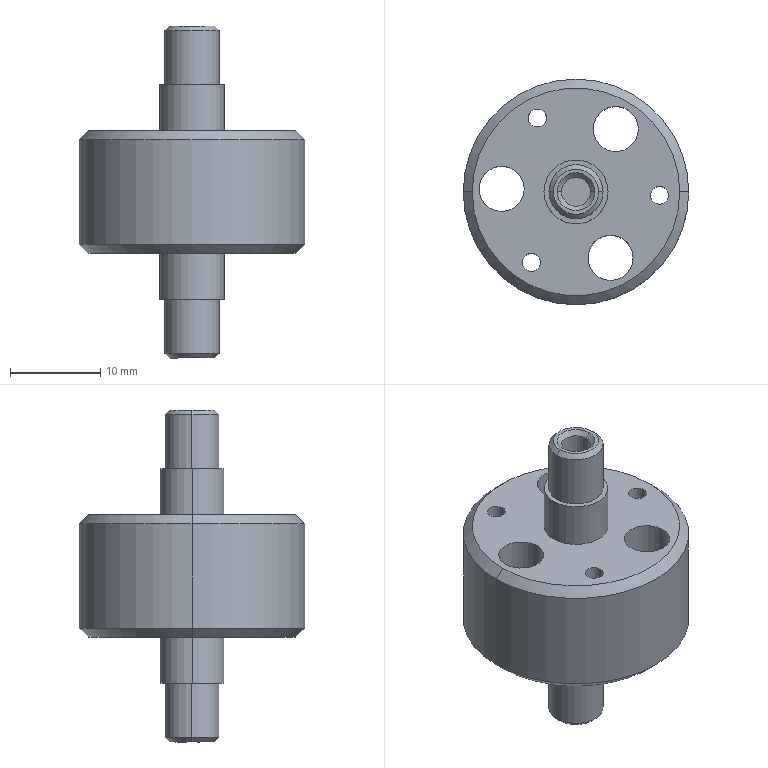Part | NX | features BREP 1 | 1 solid | 46 faces | box 25 x 25 x 36.8 mm | volume 6273 mm3 | cylinder 26 | cone 12 | plane 8 | commonest cylinder face diameters 2 x6 5 x6 3.2 x4 6 x4 7.1 x4 25 x2
STEP:
#1=CARTESIAN_POINT('',(-130.393,156.67,25.1));
#2=VERTEX_POINT('',#1);
#3=CARTESIAN_POINT('',(-127.193,156.67,25.1));
#4=VERTEX_POINT('',#3);
#5=CARTESIAN_POINT('',(-128.793,156.67,25.1));
#6=DIRECTION('',(0.,0.,1.));
#7=DIRECTION('',(1.,0.,0.));
#8=AXIS2_PLACEMENT_3D('',#5,#6,#7);
#9=CIRCLE('',#8,1.6);
#10=EDGE_CURVE('',#2,#4,#9,.T.);
#11=ORIENTED_EDGE('',*,*,#10,.F.);
#12=CARTESIAN_POINT('',(-130.893,156.67,25.6));
#13=VERTEX_POINT('',#12);
#14=CARTESIAN_POINT('',(-130.393,156.67,25.1));
#15=DIRECTION('',(-0.7071,0.,0.7071));
#16=VECTOR('',#15,1000.);
#17=LINE('',#14,#16);
#18=EDGE_CURVE('',#2,#13,#17,.T.);
#19=ORIENTED_EDGE('',*,*,#18,.T.);
#20=CARTESIAN_POINT('',(-126.693,156.67,25.6));
#21=VERTEX_POINT('',#20);
#22=CARTESIAN_POINT('',(-128.793,156.67,25.6));
#23=DIRECTION('',(0.,0.,-1.));
#24=DIRECTION('',(1.,0.,0.));
#25=AXIS2_PLACEMENT_3D('',#22,#23,#24);
#26=CIRCLE('',#25,2.1);
#27=EDGE_CURVE('',#21,#13,#26,.T.);
#28=ORIENTED_EDGE('',*,*,#27,.F.);
#29=CARTESIAN_POINT('',(-127.193,156.67,25.1));
#30=DIRECTION('',(0.7071,0.,0.7071));
#31=VECTOR('',#30,1000.);
#32=LINE('',#29,#31);
#33=EDGE_CURVE('',#4,#21,#32,.T.);
#34=ORIENTED_EDGE('',*,*,#33,.F.);
#35=EDGE_LOOP('',(#11,#19,#28,#34));
#36=FACE_BOUND('',#35,.T.);
#37=CARTESIAN_POINT('',(-128.793,156.67,25.1));
#38=DIRECTION('',(0.,0.,1.));
#39=DIRECTION('',(-1.,0.,0.));
#40=AXIS2_PLACEMENT_3D('',#37,#38,#39);
#41=CONICAL_SURFACE('',#40,1.6,0.7854);
#42=ADVANCED_FACE('',(#36),#41,.F.);
#43=CARTESIAN_POINT('',(-127.193,156.67,-10.7));
#44=VERTEX_POINT('',#43);
#45=CARTESIAN_POINT('',(-130.393,156.67,-10.7));
#46=VERTEX_POINT('',#45);
#47=CARTESIAN_POINT('',(-128.793,156.67,-10.7));
#48=DIRECTION('',(0.,0.,-1.));
#49=DIRECTION('',(1.,0.,0.));
#50=AXIS2_PLACEMENT_3D('',#47,#48,#49);
#51=CIRCLE('',#50,1.6);
#52=EDGE_CURVE('',#44,#46,#51,.T.);
#53=ORIENTED_EDGE('',*,*,#52,.F.);
#54=CARTESIAN_POINT('',(-126.693,156.67,-11.2));
#55=VERTEX_POINT('',#54);
#56=CARTESIAN_POINT('',(-127.193,156.67,-10.7));
#57=DIRECTION('',(0.7071,0.,-0.7071));
#58=VECTOR('',#57,1000.);
#59=LINE('',#56,#58);
#60=EDGE_CURVE('',#55,#44,#59,.F.);
#61=ORIENTED_EDGE('',*,*,#60,.F.);
#62=CARTESIAN_POINT('',(-130.893,156.67,-11.2));
#63=VERTEX_POINT('',#62);
#64=CARTESIAN_POINT('',(-128.793,156.67,-11.2));
#65=DIRECTION('',(0.,0.,1.));
#66=DIRECTION('',(1.,0.,0.));
#67=AXIS2_PLACEMENT_3D('',#64,#65,#66);
#68=CIRCLE('',#67,2.1);
#69=EDGE_CURVE('',#63,#55,#68,.T.);
#70=ORIENTED_EDGE('',*,*,#69,.F.);
#71=CARTESIAN_POINT('',(-130.393,156.67,-10.7));
#72=DIRECTION('',(-0.7071,0.,-0.7071));
#73=VECTOR('',#72,1000.);
#74=LINE('',#71,#73);
#75=EDGE_CURVE('',#63,#46,#74,.F.);
#76=ORIENTED_EDGE('',*,*,#75,.T.);
#77=EDGE_LOOP('',(#53,#61,#70,#76));
#78=FACE_BOUND('',#77,.T.);
#79=CARTESIAN_POINT('',(-128.793,156.67,-10.7));
#80=DIRECTION('',(0.,0.,-1.));
#81=DIRECTION('',(1.,0.,0.));
#82=AXIS2_PLACEMENT_3D('',#79,#80,#81);
#83=CONICAL_SURFACE('',#82,1.6,0.7854);
#84=ADVANCED_FACE('',(#78),#83,.F.);
#85=CARTESIAN_POINT('',(-130.393,156.67,15.6));
#86=VERTEX_POINT('',#85);
#87=CARTESIAN_POINT('',(-127.193,156.67,15.6));
#88=VERTEX_POINT('',#87);
#89=CARTESIAN_POINT('',(-128.793,156.67,15.6));
#90=DIRECTION('',(0.,0.,1.));
#91=DIRECTION('',(1.,0.,0.));
#92=AXIS2_PLACEMENT_3D('',#89,#90,#91);
#93=CIRCLE('',#92,1.6);
#94=EDGE_CURVE('',#86,#88,#93,.T.);
#95=ORIENTED_EDGE('',*,*,#94,.F.);
#96=CARTESIAN_POINT('',(-130.393,156.67,15.6));
#97=DIRECTION('',(0.,0.,1.));
#98=VECTOR('',#97,1000.);
#99=LINE('',#96,#98);
#100=EDGE_CURVE('',#86,#2,#99,.T.);
#101=ORIENTED_EDGE('',*,*,#100,.T.);
#102=ORIENTED_EDGE('',*,*,#10,.T.);
#103=CARTESIAN_POINT('',(-127.193,156.67,15.6));
#104=DIRECTION('',(0.,0.,1.));
#105=VECTOR('',#104,1000.);
#106=LINE('',#103,#105);
#107=EDGE_CURVE('',#88,#4,#106,.T.);
#108=ORIENTED_EDGE('',*,*,#107,.F.);
#109=EDGE_LOOP('',(#95,#101,#102,#108));
#110=FACE_BOUND('',#109,.T.);
#111=CARTESIAN_POINT('',(-128.793,156.67,15.6));
#112=DIRECTION('',(0.,0.,1.));
#113=DIRECTION('',(-1.,0.,0.));
#114=AXIS2_PLACEMENT_3D('',#111,#112,#113);
#115=CYLINDRICAL_SURFACE('',#114,1.6);
#116=ADVANCED_FACE('',(#110),#115,.F.);
#117=CARTESIAN_POINT('',(-127.193,156.67,-1.2));
#118=VERTEX_POINT('',#117);
#119=CARTESIAN_POINT('',(-130.393,156.67,-1.2));
#120=VERTEX_POINT('',#119);
#121=CARTESIAN_POINT('',(-128.793,156.67,-1.2));
#122=DIRECTION('',(0.,0.,-1.));
#123=DIRECTION('',(-1.,0.,0.));
#124=AXIS2_PLACEMENT_3D('',#121,#122,#123);
#125=CIRCLE('',#124,1.6);
#126=EDGE_CURVE('',#118,#120,#125,.T.);
#127=ORIENTED_EDGE('',*,*,#126,.F.);
#128=CARTESIAN_POINT('',(-127.193,156.67,-1.2));
#129=DIRECTION('',(0.,0.,-1.));
#130=VECTOR('',#129,1000.);
#131=LINE('',#128,#130);
#132=EDGE_CURVE('',#44,#118,#131,.F.);
#133=ORIENTED_EDGE('',*,*,#132,.F.);
#134=ORIENTED_EDGE('',*,*,#52,.T.);
#135=CARTESIAN_POINT('',(-130.393,156.67,-1.2));
#136=DIRECTION('',(0.,0.,-1.));
#137=VECTOR('',#136,1000.);
#138=LINE('',#135,#137);
#139=EDGE_CURVE('',#46,#120,#138,.F.);
#140=ORIENTED_EDGE('',*,*,#139,.T.);
#141=EDGE_LOOP('',(#127,#133,#134,#140));
#142=FACE_BOUND('',#141,.T.);
#143=CARTESIAN_POINT('',(-128.793,156.67,-1.2));
#144=DIRECTION('',(0.,0.,-1.));
#145=DIRECTION('',(1.,0.,0.));
#146=AXIS2_PLACEMENT_3D('',#143,#144,#145);
#147=CYLINDRICAL_SURFACE('',#146,1.6);
#148=ADVANCED_FACE('',(#142),#147,.F.);
#149=CARTESIAN_POINT('',(-126.293,156.67,25.6));
#150=VERTEX_POINT('',#149);
#151=CARTESIAN_POINT('',(-131.293,156.67,25.6));
#152=VERTEX_POINT('',#151);
#153=CARTESIAN_POINT('',(-128.793,156.67,25.6));
#154=DIRECTION('',(0.,0.,1.));
#155=DIRECTION('',(1.,0.,0.));
#156=AXIS2_PLACEMENT_3D('',#153,#154,#155);
#157=CIRCLE('',#156,2.5);
#158=EDGE_CURVE('',#150,#152,#157,.T.);
#159=ORIENTED_EDGE('',*,*,#158,.F.);
#160=CARTESIAN_POINT('',(-125.793,156.67,25.1));
#161=VERTEX_POINT('',#160);
#162=CARTESIAN_POINT('',(-126.293,156.67,25.6));
#163=DIRECTION('',(0.7071,0.,-0.7071));
#164=VECTOR('',#163,1000.);
#165=LINE('',#162,#164);
#166=EDGE_CURVE('',#161,#150,#165,.F.);
#167=ORIENTED_EDGE('',*,*,#166,.F.);
#168=CARTESIAN_POINT('',(-131.793,156.67,25.1));
#169=VERTEX_POINT('',#168);
#170=CARTESIAN_POINT('',(-128.793,156.67,25.1));
#171=DIRECTION('',(0.,0.,-1.));
#172=DIRECTION('',(1.,0.,0.));
#173=AXIS2_PLACEMENT_3D('',#170,#171,#172);
#174=CIRCLE('',#173,3.);
#175=EDGE_CURVE('',#169,#161,#174,.T.);
#176=ORIENTED_EDGE('',*,*,#175,.F.);
#177=CARTESIAN_POINT('',(-131.293,156.67,25.6));
#178=DIRECTION('',(-0.7071,0.,-0.7071));
#179=VECTOR('',#178,1000.);
#180=LINE('',#177,#179);
#181=EDGE_CURVE('',#169,#152,#180,.F.);
#182=ORIENTED_EDGE('',*,*,#181,.T.);
#183=EDGE_LOOP('',(#159,#167,#176,#182));
#184=FACE_BOUND('',#183,.T.);
#185=CARTESIAN_POINT('',(-128.793,156.67,25.6));
#186=DIRECTION('',(0.,0.,-1.));
#187=DIRECTION('',(1.,0.,0.));
#188=AXIS2_PLACEMENT_3D('',#185,#186,#187);
#189=CONICAL_SURFACE('',#188,2.5,0.7854);
#190=ADVANCED_FACE('',(#184),#189,.T.);
#191=CARTESIAN_POINT('',(-131.293,156.67,-11.2));
#192=VERTEX_POINT('',#191);
#193=CARTESIAN_POINT('',(-126.293,156.67,-11.2));
#194=VERTEX_POINT('',#193);
#195=CARTESIAN_POINT('',(-128.793,156.67,-11.2));
#196=DIRECTION('',(0.,0.,-1.));
#197=DIRECTION('',(1.,0.,0.));
#198=AXIS2_PLACEMENT_3D('',#195,#196,#197);
#199=CIRCLE('',#198,2.5);
#200=EDGE_CURVE('',#192,#194,#199,.T.);
#201=ORIENTED_EDGE('',*,*,#200,.F.);
#202=CARTESIAN_POINT('',(-131.793,156.67,-10.7));
#203=VERTEX_POINT('',#202);
#204=CARTESIAN_POINT('',(-131.293,156.67,-11.2));
#205=DIRECTION('',(-0.7071,0.,0.7071));
#206=VECTOR('',#205,1000.);
#207=LINE('',#204,#206);
#208=EDGE_CURVE('',#192,#203,#207,.T.);
#209=ORIENTED_EDGE('',*,*,#208,.T.);
#210=CARTESIAN_POINT('',(-125.793,156.67,-10.7));
#211=VERTEX_POINT('',#210);
#212=CARTESIAN_POINT('',(-128.793,156.67,-10.7));
#213=DIRECTION('',(0.,0.,1.));
#214=DIRECTION('',(1.,0.,0.));
#215=AXIS2_PLACEMENT_3D('',#212,#213,#214);
#216=CIRCLE('',#215,3.);
#217=EDGE_CURVE('',#211,#203,#216,.T.);
#218=ORIENTED_EDGE('',*,*,#217,.F.);
#219=CARTESIAN_POINT('',(-126.293,156.67,-11.2));
#220=DIRECTION('',(0.7071,0.,0.7071));
#221=VECTOR('',#220,1000.);
#222=LINE('',#219,#221);
#223=EDGE_CURVE('',#194,#211,#222,.T.);
#224=ORIENTED_EDGE('',*,*,#223,.F.);
#225=EDGE_LOOP('',(#201,#209,#218,#224));
#226=FACE_BOUND('',#225,.T.);
#227=CARTESIAN_POINT('',(-128.793,156.67,-11.2));
#228=DIRECTION('',(0.,0.,1.));
#229=DIRECTION('',(-1.,0.,0.));
#230=AXIS2_PLACEMENT_3D('',#227,#228,#229);
#231=CONICAL_SURFACE('',#230,2.5,0.7854);
#232=ADVANCED_FACE('',(#226),#231,.T.);
#233=CARTESIAN_POINT('',(-125.793,156.67,19.1));
#234=VERTEX_POINT('',#233);
#235=CARTESIAN_POINT('',(-131.793,156.67,19.1));
#236=VERTEX_POINT('',#235);
#237=CARTESIAN_POINT('',(-128.793,156.67,19.1));
#238=DIRECTION('',(0.,0.,1.));
#239=DIRECTION('',(-1.,0.,0.));
#240=AXIS2_PLACEMENT_3D('',#237,#238,#239);
#241=CIRCLE('',#240,3.);
#242=EDGE_CURVE('',#234,#236,#241,.T.);
#243=ORIENTED_EDGE('',*,*,#242,.T.);
#244=CARTESIAN_POINT('',(-131.793,156.67,-19.685));
#245=DIRECTION('',(0.,0.,1.));
#246=VECTOR('',#245,1000.);
#247=LINE('',#244,#246);
#248=EDGE_CURVE('',#236,#169,#247,.T.);
#249=ORIENTED_EDGE('',*,*,#248,.T.);
#250=ORIENTED_EDGE('',*,*,#175,.T.);
#251=CARTESIAN_POINT('',(-125.793,156.67,-19.685));
#252=DIRECTION('',(0.,0.,1.));
#253=VECTOR('',#252,1000.);
#254=LINE('',#251,#253);
#255=EDGE_CURVE('',#234,#161,#254,.T.);
#256=ORIENTED_EDGE('',*,*,#255,.F.);
#257=EDGE_LOOP('',(#243,#249,#250,#256));
#258=FACE_BOUND('',#257,.T.);
#259=CARTESIAN_POINT('',(-128.793,156.67,-19.685));
#260=DIRECTION('',(0.,0.,1.));
#261=DIRECTION('',(-1.,0.,0.));
#262=AXIS2_PLACEMENT_3D('',#259,#260,#261);
#263=CYLINDRICAL_SURFACE('',#262,3.);
#264=ADVANCED_FACE('',(#258),#263,.T.);
#265=CARTESIAN_POINT('',(-125.243,156.67,14.));
#266=VERTEX_POINT('',#265);
#267=CARTESIAN_POINT('',(-132.343,156.67,14.));
#268=VERTEX_POINT('',#267);
#269=CARTESIAN_POINT('',(-128.793,156.67,14.));
#270=DIRECTION('',(0.,0.,1.));
#271=DIRECTION('',(0.,1.,0.));
#272=AXIS2_PLACEMENT_3D('',#269,#270,#271);
#273=CIRCLE('',#272,3.55);
#274=EDGE_CURVE('',#266,#268,#273,.T.);
#275=ORIENTED_EDGE('',*,*,#274,.T.);
#276=CARTESIAN_POINT('',(-132.343,156.67,19.1));
#277=VERTEX_POINT('',#276);
#278=CARTESIAN_POINT('',(-132.343,156.67,-14.741));
#279=DIRECTION('',(0.,0.,1.));
#280=VECTOR('',#279,1000.);
#281=LINE('',#278,#280);
#282=EDGE_CURVE('',#268,#277,#281,.T.);
#283=ORIENTED_EDGE('',*,*,#282,.T.);
#284=CARTESIAN_POINT('',(-125.243,156.67,19.1));
#285=VERTEX_POINT('',#284);
#286=CARTESIAN_POINT('',(-128.793,156.67,19.1));
#287=DIRECTION('',(0.,0.,-1.));
#288=DIRECTION('',(-1.,0.,0.));
#289=AXIS2_PLACEMENT_3D('',#286,#287,#288);
#290=CIRCLE('',#289,3.55);
#291=EDGE_CURVE('',#277,#285,#290,.T.);
#292=ORIENTED_EDGE('',*,*,#291,.T.);
#293=CARTESIAN_POINT('',(-125.243,156.67,-14.741));
#294=DIRECTION('',(0.,0.,1.));
#295=VECTOR('',#294,1000.);
#296=LINE('',#293,#295);
#297=EDGE_CURVE('',#266,#285,#296,.T.);
#298=ORIENTED_EDGE('',*,*,#297,.F.);
#299=EDGE_LOOP('',(#275,#283,#292,#298));
#300=FACE_BOUND('',#299,.T.);
#301=CARTESIAN_POINT('',(-128.793,156.67,-14.741));
#302=DIRECTION('',(0.,0.,1.));
#303=DIRECTION('',(-1.,0.,0.));
#304=AXIS2_PLACEMENT_3D('',#301,#302,#303);
#305=CYLINDRICAL_SURFACE('',#304,3.55);
#306=ADVANCED_FACE('',(#300),#305,.T.);
#307=ORIENTED_EDGE('',*,*,#217,.T.);
#308=CARTESIAN_POINT('',(-131.793,156.67,-4.7));
#309=VERTEX_POINT('',#308);
#310=CARTESIAN_POINT('',(-131.793,156.67,-19.685));
#311=DIRECTION('',(0.,0.,1.));
#312=VECTOR('',#311,1000.);
#313=LINE('',#310,#312);
#314=EDGE_CURVE('',#203,#309,#313,.T.);
#315=ORIENTED_EDGE('',*,*,#314,.T.);
#316=CARTESIAN_POINT('',(-125.793,156.67,-4.7));
#317=VERTEX_POINT('',#316);
#318=CARTESIAN_POINT('',(-128.793,156.67,-4.7));
#319=DIRECTION('',(0.,0.,1.));
#320=DIRECTION('',(-1.,0.,0.));
#321=AXIS2_PLACEMENT_3D('',#318,#319,#320);
#322=CIRCLE('',#321,3.);
#323=EDGE_CURVE('',#317,#309,#322,.T.);
#324=ORIENTED_EDGE('',*,*,#323,.F.);
#325=CARTESIAN_POINT('',(-125.793,156.67,-19.685));
#326=DIRECTION('',(0.,0.,1.));
#327=VECTOR('',#326,1000.);
#328=LINE('',#325,#327);
#329=EDGE_CURVE('',#211,#317,#328,.T.);
#330=ORIENTED_EDGE('',*,*,#329,.F.);
#331=EDGE_LOOP('',(#307,#315,#324,#330));
#332=FACE_BOUND('',#331,.T.);
#333=CARTESIAN_POINT('',(-128.793,156.67,-19.685));
#334=DIRECTION('',(0.,0.,1.));
#335=DIRECTION('',(-1.,0.,0.));
#336=AXIS2_PLACEMENT_3D('',#333,#334,#335);
#337=CYLINDRICAL_SURFACE('',#336,3.);
#338=ADVANCED_FACE('',(#332),#337,.T.);
#339=CARTESIAN_POINT('',(-132.343,156.67,-4.7));
#340=VERTEX_POINT('',#339);
#341=CARTESIAN_POINT('',(-125.243,156.67,-4.7));
#342=VERTEX_POINT('',#341);
#343=CARTESIAN_POINT('',(-128.793,156.67,-4.7));
#344=DIRECTION('',(0.,0.,-1.));
#345=DIRECTION('',(-1.,0.,0.));
#346=AXIS2_PLACEMENT_3D('',#343,#344,#345);
#347=CIRCLE('',#346,3.55);
#348=EDGE_CURVE('',#340,#342,#347,.T.);
#349=ORIENTED_EDGE('',*,*,#348,.F.);
#350=CARTESIAN_POINT('',(-132.343,156.67,0.4));
#351=VERTEX_POINT('',#350);
#352=CARTESIAN_POINT('',(-132.343,156.67,-14.741));
#353=DIRECTION('',(0.,0.,1.));
#354=VECTOR('',#353,1000.);
#355=LINE('',#352,#354);
#356=EDGE_CURVE('',#340,#351,#355,.T.);
#357=ORIENTED_EDGE('',*,*,#356,.T.);
#358=CARTESIAN_POINT('',(-125.243,156.67,0.4));
#359=VERTEX_POINT('',#358);
#360=CARTESIAN_POINT('',(-128.793,156.67,0.4));
#361=DIRECTION('',(0.,0.,-1.));
#362=DIRECTION('',(1.,0.,0.));
#363=AXIS2_PLACEMENT_3D('',#360,#361,#362);
#364=CIRCLE('',#363,3.55);
#365=EDGE_CURVE('',#351,#359,#364,.T.);
#366=ORIENTED_EDGE('',*,*,#365,.T.);
#367=CARTESIAN_POINT('',(-125.243,156.67,-14.741));
#368=DIRECTION('',(0.,0.,1.));
#369=VECTOR('',#368,1000.);
#370=LINE('',#367,#369);
#371=EDGE_CURVE('',#342,#359,#370,.T.);
#372=ORIENTED_EDGE('',*,*,#371,.F.);
#373=EDGE_LOOP('',(#349,#357,#366,#372));
#374=FACE_BOUND('',#373,.T.);
#375=CARTESIAN_POINT('',(-128.793,156.67,-14.741));
#376=DIRECTION('',(0.,0.,1.));
#377=DIRECTION('',(-1.,0.,0.));
#378=AXIS2_PLACEMENT_3D('',#375,#376,#377);
#379=CYLINDRICAL_SURFACE('',#378,3.55);
#380=ADVANCED_FACE('',(#374),#379,.T.);
#381=CARTESIAN_POINT('',(-126.88,163.64,0.4));
#382=VERTEX_POINT('',#381);
#383=CARTESIAN_POINT('',(-121.88,163.64,0.4));
#384=VERTEX_POINT('',#383);
#385=CARTESIAN_POINT('',(-124.38,163.64,0.4));
#386=DIRECTION('',(0.,0.,1.));
#387=DIRECTION('',(1.,0.,0.));
#388=AXIS2_PLACEMENT_3D('',#385,#386,#387);
#389=CIRCLE('',#388,2.5);
#390=EDGE_CURVE('',#382,#384,#389,.T.);
#391=ORIENTED_EDGE('',*,*,#390,.F.);
#392=CARTESIAN_POINT('',(-126.88,163.64,14.));
#393=VERTEX_POINT('',#392);
#394=CARTESIAN_POINT('',(-126.88,163.64,-4.));
#395=DIRECTION('',(0.,0.,1.));
#396=VECTOR('',#395,1000.);
#397=LINE('',#394,#396);
#398=EDGE_CURVE('',#382,#393,#397,.T.);
#399=ORIENTED_EDGE('',*,*,#398,.T.);
#400=CARTESIAN_POINT('',(-121.88,163.64,14.));
#401=VERTEX_POINT('',#400);
#402=CARTESIAN_POINT('',(-124.38,163.64,14.));
#403=DIRECTION('',(0.,0.,1.));
#404=DIRECTION('',(1.,0.,0.));
#405=AXIS2_PLACEMENT_3D('',#402,#403,#404);
#406=CIRCLE('',#405,2.5);
#407=EDGE_CURVE('',#393,#401,#406,.T.);
#408=ORIENTED_EDGE('',*,*,#407,.T.);
#409=CARTESIAN_POINT('',(-121.88,163.64,-4.));
#410=DIRECTION('',(0.,0.,1.));
#411=VECTOR('',#410,1000.);
#412=LINE('',#409,#411);
#413=EDGE_CURVE('',#384,#401,#412,.T.);
#414=ORIENTED_EDGE('',*,*,#413,.F.);
#415=EDGE_LOOP('',(#391,#399,#408,#414));
#416=FACE_BOUND('',#415,.T.);
#417=CARTESIAN_POINT('',(-124.38,163.64,-4.));
#418=DIRECTION('',(0.,0.,1.));
#419=DIRECTION('',(-1.,0.,0.));
#420=AXIS2_PLACEMENT_3D('',#417,#418,#419);
#421=CYLINDRICAL_SURFACE('',#420,2.5);
#422=ADVANCED_FACE('',(#416),#421,.F.);
#423=CARTESIAN_POINT('',(-127.463,149.363,0.4));
#424=VERTEX_POINT('',#423);
#425=CARTESIAN_POINT('',(-122.463,149.363,0.4));
#426=VERTEX_POINT('',#425);
#427=CARTESIAN_POINT('',(-124.963,149.363,0.4));
#428=DIRECTION('',(0.,0.,1.));
#429=DIRECTION('',(1.,0.,0.));
#430=AXIS2_PLACEMENT_3D('',#427,#428,#429);
#431=CIRCLE('',#430,2.5);
#432=EDGE_CURVE('',#424,#426,#431,.T.);
#433=ORIENTED_EDGE('',*,*,#432,.F.);
#434=CARTESIAN_POINT('',(-127.463,149.363,14.));
#435=VERTEX_POINT('',#434);
#436=CARTESIAN_POINT('',(-127.463,149.363,-4.));
#437=DIRECTION('',(0.,0.,1.));
#438=VECTOR('',#437,1000.);
#439=LINE('',#436,#438);
#440=EDGE_CURVE('',#424,#435,#439,.T.);
#441=ORIENTED_EDGE('',*,*,#440,.T.);
#442=CARTESIAN_POINT('',(-122.463,149.363,14.));
#443=VERTEX_POINT('',#442);
#444=CARTESIAN_POINT('',(-124.963,149.363,14.));
#445=DIRECTION('',(0.,0.,1.));
#446=DIRECTION('',(1.,0.,0.));
#447=AXIS2_PLACEMENT_3D('',#444,#445,#446);
#448=CIRCLE('',#447,2.5);
#449=EDGE_CURVE('',#435,#443,#448,.T.);
#450=ORIENTED_EDGE('',*,*,#449,.T.);
#451=CARTESIAN_POINT('',(-122.463,149.363,-4.));
#452=DIRECTION('',(0.,0.,1.));
#453=VECTOR('',#452,1000.);
#454=LINE('',#451,#453);
#455=EDGE_CURVE('',#426,#443,#454,.T.);
#456=ORIENTED_EDGE('',*,*,#455,.F.);
#457=EDGE_LOOP('',(#433,#441,#450,#456));
#458=FACE_BOUND('',#457,.T.);
#459=CARTESIAN_POINT('',(-124.963,149.363,-4.));
#460=DIRECTION('',(0.,0.,1.));
#461=DIRECTION('',(-1.,0.,0.));
#462=AXIS2_PLACEMENT_3D('',#459,#460,#461);
#463=CYLINDRICAL_SURFACE('',#462,2.5);
#464=ADVANCED_FACE('',(#458),#463,.F.);
#465=CARTESIAN_POINT('',(-139.536,157.006,0.4));
#466=VERTEX_POINT('',#465);
#467=CARTESIAN_POINT('',(-134.536,157.006,0.4));
#468=VERTEX_POINT('',#467);
#469=CARTESIAN_POINT('',(-137.036,157.006,0.4));
#470=DIRECTION('',(0.,0.,1.));
#471=DIRECTION('',(1.,0.,0.));
#472=AXIS2_PLACEMENT_3D('',#469,#470,#471);
#473=CIRCLE('',#472,2.5);
#474=EDGE_CURVE('',#466,#468,#473,.T.);
#475=ORIENTED_EDGE('',*,*,#474,.F.);
#476=CARTESIAN_POINT('',(-139.536,157.006,14.));
#477=VERTEX_POINT('',#476);
#478=CARTESIAN_POINT('',(-139.536,157.006,-4.));
#479=DIRECTION('',(0.,0.,1.));
#480=VECTOR('',#479,1000.);
#481=LINE('',#478,#480);
#482=EDGE_CURVE('',#466,#477,#481,.T.);
#483=ORIENTED_EDGE('',*,*,#482,.T.);
#484=CARTESIAN_POINT('',(-134.536,157.006,14.));
#485=VERTEX_POINT('',#484);
#486=CARTESIAN_POINT('',(-137.036,157.006,14.));
#487=DIRECTION('',(0.,0.,1.));
#488=DIRECTION('',(1.,0.,0.));
#489=AXIS2_PLACEMENT_3D('',#486,#487,#488);
#490=CIRCLE('',#489,2.5);
#491=EDGE_CURVE('',#477,#485,#490,.T.);
#492=ORIENTED_EDGE('',*,*,#491,.T.);
#493=CARTESIAN_POINT('',(-134.536,157.006,-4.));
#494=DIRECTION('',(0.,0.,1.));
#495=VECTOR('',#494,1000.);
#496=LINE('',#493,#495);
#497=EDGE_CURVE('',#468,#485,#496,.T.);
#498=ORIENTED_EDGE('',*,*,#497,.F.);
#499=EDGE_LOOP('',(#475,#483,#492,#498));
#500=FACE_BOUND('',#499,.T.);
#501=CARTESIAN_POINT('',(-137.036,157.006,-4.));
#502=DIRECTION('',(0.,0.,1.));
#503=DIRECTION('',(-1.,0.,0.));
#504=AXIS2_PLACEMENT_3D('',#501,#502,#503);
#505=CYLINDRICAL_SURFACE('',#504,2.5);
#506=ADVANCED_FACE('',(#500),#505,.F.);
#507=CARTESIAN_POINT('',(-117.293,156.67,14.));
#508=VERTEX_POINT('',#507);
#509=CARTESIAN_POINT('',(-140.293,156.67,14.));
#510=VERTEX_POINT('',#509);
#511=CARTESIAN_POINT('',(-128.793,156.67,14.));
#512=DIRECTION('',(0.,0.,1.));
#513=DIRECTION('',(0.,1.,0.));
#514=AXIS2_PLACEMENT_3D('',#511,#512,#513);
#515=CIRCLE('',#514,11.5);
#516=EDGE_CURVE('',#508,#510,#515,.T.);
#517=ORIENTED_EDGE('',*,*,#516,.F.);
#518=CARTESIAN_POINT('',(-116.293,156.67,13.));
#519=VERTEX_POINT('',#518);
#520=CARTESIAN_POINT('',(-116.293,156.67,13.));
#521=DIRECTION('',(0.7071,0.,-0.7071));
#522=VECTOR('',#521,1000.);
#523=LINE('',#520,#522);
#524=EDGE_CURVE('',#519,#508,#523,.F.);
#525=ORIENTED_EDGE('',*,*,#524,.F.);
#526=CARTESIAN_POINT('',(-141.293,156.67,13.));
#527=VERTEX_POINT('',#526);
#528=CARTESIAN_POINT('',(-128.793,156.67,13.));
#529=DIRECTION('',(0.,0.,-1.));
#530=DIRECTION('',(-1.,0.,0.));
#531=AXIS2_PLACEMENT_3D('',#528,#529,#530);
#532=CIRCLE('',#531,12.5);
#533=EDGE_CURVE('',#527,#519,#532,.T.);
#534=ORIENTED_EDGE('',*,*,#533,.F.);
#535=CARTESIAN_POINT('',(-141.293,156.67,13.));
#536=DIRECTION('',(-0.7071,0.,-0.7071));
#537=VECTOR('',#536,1000.);
#538=LINE('',#535,#537);
#539=EDGE_CURVE('',#527,#510,#538,.F.);
#540=ORIENTED_EDGE('',*,*,#539,.T.);
#541=EDGE_LOOP('',(#517,#525,#534,#540));
#542=FACE_BOUND('',#541,.T.);
#543=CARTESIAN_POINT('',(-128.793,156.67,13.));
#544=DIRECTION('',(0.,0.,-1.));
#545=DIRECTION('',(1.,0.,0.));
#546=AXIS2_PLACEMENT_3D('',#543,#544,#545);
#547=CONICAL_SURFACE('',#546,12.5,0.7854);
#548=ADVANCED_FACE('',(#542),#547,.T.);
#549=CARTESIAN_POINT('',(-140.293,156.67,0.4));
#550=VERTEX_POINT('',#549);
#551=CARTESIAN_POINT('',(-117.293,156.67,0.4));
#552=VERTEX_POINT('',#551);
#553=CARTESIAN_POINT('',(-128.793,156.67,0.4));
#554=DIRECTION('',(0.,0.,-1.));
#555=DIRECTION('',(1.,0.,0.));
#556=AXIS2_PLACEMENT_3D('',#553,#554,#555);
#557=CIRCLE('',#556,11.5);
#558=EDGE_CURVE('',#550,#552,#557,.T.);
#559=ORIENTED_EDGE('',*,*,#558,.F.);
#560=CARTESIAN_POINT('',(-141.293,156.67,1.4));
#561=VERTEX_POINT('',#560);
#562=CARTESIAN_POINT('',(-141.293,156.67,1.4));
#563=DIRECTION('',(-0.7071,0.,0.7071));
#564=VECTOR('',#563,1000.);
#565=LINE('',#562,#564);
#566=EDGE_CURVE('',#550,#561,#565,.T.);
#567=ORIENTED_EDGE('',*,*,#566,.T.);
#568=CARTESIAN_POINT('',(-116.293,156.67,1.4));
#569=VERTEX_POINT('',#568);
#570=CARTESIAN_POINT('',(-128.793,156.67,1.4));
#571=DIRECTION('',(0.,0.,1.));
#572=DIRECTION('',(1.,0.,0.));
#573=AXIS2_PLACEMENT_3D('',#570,#571,#572);
#574=CIRCLE('',#573,12.5);
#575=EDGE_CURVE('',#569,#561,#574,.T.);
#576=ORIENTED_EDGE('',*,*,#575,.F.);
#577=CARTESIAN_POINT('',(-116.293,156.67,1.4));
#578=DIRECTION('',(0.7071,0.,0.7071));
#579=VECTOR('',#578,1000.);
#580=LINE('',#577,#579);
#581=EDGE_CURVE('',#552,#569,#580,.T.);
#582=ORIENTED_EDGE('',*,*,#581,.F.);
#583=EDGE_LOOP('',(#559,#567,#576,#582));
#584=FACE_BOUND('',#583,.T.);
#585=CARTESIAN_POINT('',(-128.793,156.67,1.4));
#586=DIRECTION('',(0.,0.,1.));
#587=DIRECTION('',(-1.,0.,0.));
#588=AXIS2_PLACEMENT_3D('',#585,#586,#587);
#589=CONICAL_SURFACE('',#588,12.5,0.7854);
#590=ADVANCED_FACE('',(#584),#589,.T.);
#591=CARTESIAN_POINT('',(-134.088,164.862,0.4));
#592=VERTEX_POINT('',#591);
#593=CARTESIAN_POINT('',(-132.088,164.862,0.4));
#594=VERTEX_POINT('',#593);
#595=CARTESIAN_POINT('',(-133.088,164.862,0.4));
#596=DIRECTION('',(0.,0.,1.));
#597=DIRECTION('',(1.,0.,0.));
#598=AXIS2_PLACEMENT_3D('',#595,#596,#597);
#599=CIRCLE('',#598,1.);
#600=EDGE_CURVE('',#592,#594,#599,.T.);
#601=ORIENTED_EDGE('',*,*,#600,.F.);
#602=CARTESIAN_POINT('',(-134.088,164.862,14.));
#603=VERTEX_POINT('',#602);
#604=CARTESIAN_POINT('',(-134.088,164.862,-15.));
#605=DIRECTION('',(0.,0.,1.));
#606=VECTOR('',#605,1000.);
#607=LINE('',#604,#606);
#608=EDGE_CURVE('',#592,#603,#607,.T.);
#609=ORIENTED_EDGE('',*,*,#608,.T.);
#610=CARTESIAN_POINT('',(-132.088,164.862,14.));
#611=VERTEX_POINT('',#610);
#612=CARTESIAN_POINT('',(-133.088,164.862,14.));
#613=DIRECTION('',(0.,0.,1.));
#614=DIRECTION('',(1.,0.,0.));
#615=AXIS2_PLACEMENT_3D('',#612,#613,#614);
#616=CIRCLE('',#615,1.);
#617=EDGE_CURVE('',#603,#611,#616,.T.);
#618=ORIENTED_EDGE('',*,*,#617,.T.);
#619=CARTESIAN_POINT('',(-132.088,164.862,-15.));
#620=DIRECTION('',(0.,0.,1.));
#621=VECTOR('',#620,1000.);
#622=LINE('',#619,#621);
#623=EDGE_CURVE('',#594,#611,#622,.T.);
#624=ORIENTED_EDGE('',*,*,#623,.F.);
#625=EDGE_LOOP('',(#601,#609,#618,#624));
#626=FACE_BOUND('',#625,.T.);
#627=CARTESIAN_POINT('',(-133.088,164.862,-15.));
#628=DIRECTION('',(0.,0.,1.));
#629=DIRECTION('',(-1.,0.,0.));
#630=AXIS2_PLACEMENT_3D('',#627,#628,#629);
#631=CYLINDRICAL_SURFACE('',#630,1.);
#632=ADVANCED_FACE('',(#626),#631,.F.);
#633=CARTESIAN_POINT('',(-134.741,148.854,0.4));
#634=VERTEX_POINT('',#633);
#635=CARTESIAN_POINT('',(-132.741,148.854,0.4));
#636=VERTEX_POINT('',#635);
#637=CARTESIAN_POINT('',(-133.741,148.854,0.4));
#638=DIRECTION('',(0.,0.,1.));
#639=DIRECTION('',(1.,0.,0.));
#640=AXIS2_PLACEMENT_3D('',#637,#638,#639);
#641=CIRCLE('',#640,1.);
#642=EDGE_CURVE('',#634,#636,#641,.T.);
#643=ORIENTED_EDGE('',*,*,#642,.F.);
#644=CARTESIAN_POINT('',(-134.741,148.854,14.));
#645=VERTEX_POINT('',#644);
#646=CARTESIAN_POINT('',(-134.741,148.854,-15.));
#647=DIRECTION('',(0.,0.,1.));
#648=VECTOR('',#647,1000.);
#649=LINE('',#646,#648);
#650=EDGE_CURVE('',#634,#645,#649,.T.);
#651=ORIENTED_EDGE('',*,*,#650,.T.);
#652=CARTESIAN_POINT('',(-132.741,148.854,14.));
#653=VERTEX_POINT('',#652);
#654=CARTESIAN_POINT('',(-133.741,148.854,14.));
#655=DIRECTION('',(0.,0.,1.));
#656=DIRECTION('',(1.,0.,0.));
#657=AXIS2_PLACEMENT_3D('',#654,#655,#656);
#658=CIRCLE('',#657,1.);
#659=EDGE_CURVE('',#645,#653,#658,.T.);
#660=ORIENTED_EDGE('',*,*,#659,.T.);
#661=CARTESIAN_POINT('',(-132.741,148.854,-15.));
#662=DIRECTION('',(0.,0.,1.));
#663=VECTOR('',#662,1000.);
#664=LINE('',#661,#663);
#665=EDGE_CURVE('',#636,#653,#664,.T.);
#666=ORIENTED_EDGE('',*,*,#665,.F.);
#667=EDGE_LOOP('',(#643,#651,#660,#666));
#668=FACE_BOUND('',#667,.T.);
#669=CARTESIAN_POINT('',(-133.741,148.854,-15.));
#670=DIRECTION('',(0.,0.,1.));
#671=DIRECTION('',(-1.,0.,0.));
#672=AXIS2_PLACEMENT_3D('',#669,#670,#671);
#673=CYLINDRICAL_SURFACE('',#672,1.);
#674=ADVANCED_FACE('',(#668),#673,.F.);
#675=CARTESIAN_POINT('',(-120.551,156.293,0.4));
#676=VERTEX_POINT('',#675);
#677=CARTESIAN_POINT('',(-118.551,156.293,0.4));
#678=VERTEX_POINT('',#677);
#679=CARTESIAN_POINT('',(-119.551,156.293,0.4));
#680=DIRECTION('',(0.,0.,1.));
#681=DIRECTION('',(1.,0.,0.));
#682=AXIS2_PLACEMENT_3D('',#679,#680,#681);
#683=CIRCLE('',#682,1.);
#684=EDGE_CURVE('',#676,#678,#683,.T.);
#685=ORIENTED_EDGE('',*,*,#684,.F.);
#686=CARTESIAN_POINT('',(-120.551,156.293,14.));
#687=VERTEX_POINT('',#686);
#688=CARTESIAN_POINT('',(-120.551,156.293,-15.));
#689=DIRECTION('',(0.,0.,1.));
#690=VECTOR('',#689,1000.);
#691=LINE('',#688,#690);
#692=EDGE_CURVE('',#676,#687,#691,.T.);
#693=ORIENTED_EDGE('',*,*,#692,.T.);
#694=CARTESIAN_POINT('',(-118.551,156.293,14.));
#695=VERTEX_POINT('',#694);
#696=CARTESIAN_POINT('',(-119.551,156.293,14.));
#697=DIRECTION('',(0.,0.,1.));
#698=DIRECTION('',(1.,0.,0.));
#699=AXIS2_PLACEMENT_3D('',#696,#697,#698);
#700=CIRCLE('',#699,1.);
#701=EDGE_CURVE('',#687,#695,#700,.T.);
#702=ORIENTED_EDGE('',*,*,#701,.T.);
#703=CARTESIAN_POINT('',(-118.551,156.293,-15.));
#704=DIRECTION('',(0.,0.,1.));
#705=VECTOR('',#704,1000.);
#706=LINE('',#703,#705);
#707=EDGE_CURVE('',#678,#695,#706,.T.);
#708=ORIENTED_EDGE('',*,*,#707,.F.);
#709=EDGE_LOOP('',(#685,#693,#702,#708));
#710=FACE_BOUND('',#709,.T.);
#711=CARTESIAN_POINT('',(-119.551,156.293,-15.));
#712=DIRECTION('',(0.,0.,1.));
#713=DIRECTION('',(-1.,0.,0.));
#714=AXIS2_PLACEMENT_3D('',#711,#712,#713);
#715=CYLINDRICAL_SURFACE('',#714,1.);
#716=ADVANCED_FACE('',(#710),#715,.F.);
#717=ORIENTED_EDGE('',*,*,#533,.T.);
#718=CARTESIAN_POINT('',(-116.293,156.67,49.355));
#719=DIRECTION('',(0.,0.,-1.));
#720=VECTOR('',#719,1000.);
#721=LINE('',#718,#720);
#722=EDGE_CURVE('',#569,#519,#721,.F.);
#723=ORIENTED_EDGE('',*,*,#722,.F.);
#724=ORIENTED_EDGE('',*,*,#575,.T.);
#725=CARTESIAN_POINT('',(-141.293,156.67,49.355));
#726=DIRECTION('',(0.,0.,-1.));
#727=VECTOR('',#726,1000.);
#728=LINE('',#725,#727);
#729=EDGE_CURVE('',#561,#527,#728,.F.);
#730=ORIENTED_EDGE('',*,*,#729,.T.);
#731=EDGE_LOOP('',(#717,#723,#724,#730));
#732=FACE_BOUND('',#731,.T.);
#733=CARTESIAN_POINT('',(-128.793,156.67,49.355));
#734=DIRECTION('',(0.,0.,-1.));
#735=DIRECTION('',(1.,0.,0.));
#736=AXIS2_PLACEMENT_3D('',#733,#734,#735);
#737=CYLINDRICAL_SURFACE('',#736,12.5);
#738=ADVANCED_FACE('',(#732),#737,.T.);
#739=CARTESIAN_POINT('',(-128.793,156.67,0.4));
#740=DIRECTION('',(0.,0.,-1.));
#741=DIRECTION('',(1.,0.,0.));
#742=AXIS2_PLACEMENT_3D('',#739,#740,#741);
#743=CIRCLE('',#742,11.5);
#744=EDGE_CURVE('',#552,#550,#743,.T.);
#745=ORIENTED_EDGE('',*,*,#744,.T.);
#746=ORIENTED_EDGE('',*,*,#558,.T.);
#747=EDGE_LOOP('',(#745,#746));
#748=FACE_BOUND('',#747,.T.);
#749=CARTESIAN_POINT('',(-128.793,156.67,0.4));
#750=DIRECTION('',(0.,0.,-1.));
#751=DIRECTION('',(1.,0.,0.));
#752=AXIS2_PLACEMENT_3D('',#749,#750,#751);
#753=CIRCLE('',#752,3.55);
#754=EDGE_CURVE('',#359,#351,#753,.T.);
#755=ORIENTED_EDGE('',*,*,#754,.F.);
#756=ORIENTED_EDGE('',*,*,#365,.F.);
#757=EDGE_LOOP('',(#755,#756));
#758=FACE_BOUND('',#757,.T.);
#759=CARTESIAN_POINT('',(-124.38,163.64,0.4));
#760=DIRECTION('',(0.,0.,1.));
#761=DIRECTION('',(1.,0.,0.));
#762=AXIS2_PLACEMENT_3D('',#759,#760,#761);
#763=CIRCLE('',#762,2.5);
#764=EDGE_CURVE('',#384,#382,#763,.T.);
#765=ORIENTED_EDGE('',*,*,#764,.T.);
#766=ORIENTED_EDGE('',*,*,#390,.T.);
#767=EDGE_LOOP('',(#765,#766));
#768=FACE_BOUND('',#767,.T.);
#769=CARTESIAN_POINT('',(-124.963,149.363,0.4));
#770=DIRECTION('',(0.,0.,1.));
#771=DIRECTION('',(1.,0.,0.));
#772=AXIS2_PLACEMENT_3D('',#769,#770,#771);
#773=CIRCLE('',#772,2.5);
#774=EDGE_CURVE('',#426,#424,#773,.T.);
#775=ORIENTED_EDGE('',*,*,#774,.T.);
#776=ORIENTED_EDGE('',*,*,#432,.T.);
#777=EDGE_LOOP('',(#775,#776));
#778=FACE_BOUND('',#777,.T.);
#779=CARTESIAN_POINT('',(-137.036,157.006,0.4));
#780=DIRECTION('',(0.,0.,1.));
#781=DIRECTION('',(1.,0.,0.));
#782=AXIS2_PLACEMENT_3D('',#779,#780,#781);
#783=CIRCLE('',#782,2.5);
#784=EDGE_CURVE('',#468,#466,#783,.T.);
#785=ORIENTED_EDGE('',*,*,#784,.T.);
#786=ORIENTED_EDGE('',*,*,#474,.T.);
#787=EDGE_LOOP('',(#785,#786));
#788=FACE_BOUND('',#787,.T.);
#789=CARTESIAN_POINT('',(-133.088,164.862,0.4));
#790=DIRECTION('',(0.,0.,1.));
#791=DIRECTION('',(1.,0.,0.));
#792=AXIS2_PLACEMENT_3D('',#789,#790,#791);
#793=CIRCLE('',#792,1.);
#794=EDGE_CURVE('',#594,#592,#793,.T.);
#795=ORIENTED_EDGE('',*,*,#794,.T.);
#796=ORIENTED_EDGE('',*,*,#600,.T.);
#797=EDGE_LOOP('',(#795,#796));
#798=FACE_BOUND('',#797,.T.);
#799=CARTESIAN_POINT('',(-133.741,148.854,0.4));
#800=DIRECTION('',(0.,0.,1.));
#801=DIRECTION('',(1.,0.,0.));
#802=AXIS2_PLACEMENT_3D('',#799,#800,#801);
#803=CIRCLE('',#802,1.);
#804=EDGE_CURVE('',#636,#634,#803,.T.);
#805=ORIENTED_EDGE('',*,*,#804,.T.);
#806=ORIENTED_EDGE('',*,*,#642,.T.);
#807=EDGE_LOOP('',(#805,#806));
#808=FACE_BOUND('',#807,.T.);
#809=CARTESIAN_POINT('',(-119.551,156.293,0.4));
#810=DIRECTION('',(0.,0.,1.));
#811=DIRECTION('',(1.,0.,0.));
#812=AXIS2_PLACEMENT_3D('',#809,#810,#811);
#813=CIRCLE('',#812,1.);
#814=EDGE_CURVE('',#678,#676,#813,.T.);
#815=ORIENTED_EDGE('',*,*,#814,.T.);
#816=ORIENTED_EDGE('',*,*,#684,.T.);
#817=EDGE_LOOP('',(#815,#816));
#818=FACE_BOUND('',#817,.T.);
#819=CARTESIAN_POINT('',(-128.793,156.67,0.4));
#820=DIRECTION('',(0.,0.,1.));
#821=DIRECTION('',(-1.,0.,0.));
#822=AXIS2_PLACEMENT_3D('',#819,#820,#821);
#823=PLANE('',#822);
#824=ADVANCED_FACE('',(#748,#758,#768,#778,#788,#798,#808,#818),#823,.F.);
#825=ORIENTED_EDGE('',*,*,#722,.T.);
#826=CARTESIAN_POINT('',(-128.793,156.67,13.));
#827=DIRECTION('',(0.,0.,-1.));
#828=DIRECTION('',(-1.,0.,0.));
#829=AXIS2_PLACEMENT_3D('',#826,#827,#828);
#830=CIRCLE('',#829,12.5);
#831=EDGE_CURVE('',#519,#527,#830,.T.);
#832=ORIENTED_EDGE('',*,*,#831,.T.);
#833=ORIENTED_EDGE('',*,*,#729,.F.);
#834=CARTESIAN_POINT('',(-128.793,156.67,1.4));
#835=DIRECTION('',(0.,0.,1.));
#836=DIRECTION('',(1.,0.,0.));
#837=AXIS2_PLACEMENT_3D('',#834,#835,#836);
#838=CIRCLE('',#837,12.5);
#839=EDGE_CURVE('',#561,#569,#838,.T.);
#840=ORIENTED_EDGE('',*,*,#839,.T.);
#841=EDGE_LOOP('',(#825,#832,#833,#840));
#842=FACE_BOUND('',#841,.T.);
#843=CARTESIAN_POINT('',(-128.793,156.67,49.355));
#844=DIRECTION('',(0.,0.,-1.));
#845=DIRECTION('',(1.,0.,0.));
#846=AXIS2_PLACEMENT_3D('',#843,#844,#845);
#847=CYLINDRICAL_SURFACE('',#846,12.5);
#848=ADVANCED_FACE('',(#842),#847,.T.);
#849=CARTESIAN_POINT('',(-128.793,156.67,14.));
#850=DIRECTION('',(0.,0.,1.));
#851=DIRECTION('',(0.,1.,0.));
#852=AXIS2_PLACEMENT_3D('',#849,#850,#851);
#853=CIRCLE('',#852,11.5);
#854=EDGE_CURVE('',#510,#508,#853,.T.);
#855=ORIENTED_EDGE('',*,*,#854,.T.);
#856=ORIENTED_EDGE('',*,*,#516,.T.);
#857=EDGE_LOOP('',(#855,#856));
#858=FACE_BOUND('',#857,.T.);
#859=ORIENTED_EDGE('',*,*,#274,.F.);
#860=CARTESIAN_POINT('',(-128.793,156.67,14.));
#861=DIRECTION('',(0.,0.,1.));
#862=DIRECTION('',(0.,1.,0.));
#863=AXIS2_PLACEMENT_3D('',#860,#861,#862);
#864=CIRCLE('',#863,3.55);
#865=EDGE_CURVE('',#268,#266,#864,.T.);
#866=ORIENTED_EDGE('',*,*,#865,.F.);
#867=EDGE_LOOP('',(#859,#866));
#868=FACE_BOUND('',#867,.T.);
#869=CARTESIAN_POINT('',(-124.38,163.64,14.));
#870=DIRECTION('',(0.,0.,1.));
#871=DIRECTION('',(1.,0.,0.));
#872=AXIS2_PLACEMENT_3D('',#869,#870,#871);
#873=CIRCLE('',#872,2.5);
#874=EDGE_CURVE('',#401,#393,#873,.T.);
#875=ORIENTED_EDGE('',*,*,#874,.F.);
#876=ORIENTED_EDGE('',*,*,#407,.F.);
#877=EDGE_LOOP('',(#875,#876));
#878=FACE_BOUND('',#877,.T.);
#879=CARTESIAN_POINT('',(-124.963,149.363,14.));
#880=DIRECTION('',(0.,0.,1.));
#881=DIRECTION('',(1.,0.,0.));
#882=AXIS2_PLACEMENT_3D('',#879,#880,#881);
#883=CIRCLE('',#882,2.5);
#884=EDGE_CURVE('',#443,#435,#883,.T.);
#885=ORIENTED_EDGE('',*,*,#884,.F.);
#886=ORIENTED_EDGE('',*,*,#449,.F.);
#887=EDGE_LOOP('',(#885,#886));
#888=FACE_BOUND('',#887,.T.);
#889=CARTESIAN_POINT('',(-137.036,157.006,14.));
#890=DIRECTION('',(0.,0.,1.));
#891=DIRECTION('',(1.,0.,0.));
#892=AXIS2_PLACEMENT_3D('',#889,#890,#891);
#893=CIRCLE('',#892,2.5);
#894=EDGE_CURVE('',#485,#477,#893,.T.);
#895=ORIENTED_EDGE('',*,*,#894,.F.);
#896=ORIENTED_EDGE('',*,*,#491,.F.);
#897=EDGE_LOOP('',(#895,#896));
#898=FACE_BOUND('',#897,.T.);
#899=CARTESIAN_POINT('',(-133.088,164.862,14.));
#900=DIRECTION('',(0.,0.,1.));
#901=DIRECTION('',(1.,0.,0.));
#902=AXIS2_PLACEMENT_3D('',#899,#900,#901);
#903=CIRCLE('',#902,1.);
#904=EDGE_CURVE('',#611,#603,#903,.T.);
#905=ORIENTED_EDGE('',*,*,#904,.F.);
#906=ORIENTED_EDGE('',*,*,#617,.F.);
#907=EDGE_LOOP('',(#905,#906));
#908=FACE_BOUND('',#907,.T.);
#909=CARTESIAN_POINT('',(-133.741,148.854,14.));
#910=DIRECTION('',(0.,0.,1.));
#911=DIRECTION('',(1.,0.,0.));
#912=AXIS2_PLACEMENT_3D('',#909,#910,#911);
#913=CIRCLE('',#912,1.);
#914=EDGE_CURVE('',#653,#645,#913,.T.);
#915=ORIENTED_EDGE('',*,*,#914,.F.);
#916=ORIENTED_EDGE('',*,*,#659,.F.);
#917=EDGE_LOOP('',(#915,#916));
#918=FACE_BOUND('',#917,.T.);
#919=CARTESIAN_POINT('',(-119.551,156.293,14.));
#920=DIRECTION('',(0.,0.,1.));
#921=DIRECTION('',(1.,0.,0.));
#922=AXIS2_PLACEMENT_3D('',#919,#920,#921);
#923=CIRCLE('',#922,1.);
#924=EDGE_CURVE('',#695,#687,#923,.T.);
#925=ORIENTED_EDGE('',*,*,#924,.F.);
#926=ORIENTED_EDGE('',*,*,#701,.F.);
#927=EDGE_LOOP('',(#925,#926));
#928=FACE_BOUND('',#927,.T.);
#929=CARTESIAN_POINT('',(4.059,226.313,14.));
#930=DIRECTION('',(0.,0.,-1.));
#931=DIRECTION('',(1.,0.,0.));
#932=AXIS2_PLACEMENT_3D('',#929,#930,#931);
#933=PLANE('',#932);
#934=ADVANCED_FACE('',(#858,#868,#878,#888,#898,#908,#918,#928),#933,.F.);
#935=ORIENTED_EDGE('',*,*,#692,.F.);
#936=ORIENTED_EDGE('',*,*,#814,.F.);
#937=ORIENTED_EDGE('',*,*,#707,.T.);
#938=ORIENTED_EDGE('',*,*,#924,.T.);
#939=EDGE_LOOP('',(#935,#936,#937,#938));
#940=FACE_BOUND('',#939,.T.);
#941=CARTESIAN_POINT('',(-119.551,156.293,-15.));
#942=DIRECTION('',(0.,0.,1.));
#943=DIRECTION('',(-1.,0.,0.));
#944=AXIS2_PLACEMENT_3D('',#941,#942,#943);
#945=CYLINDRICAL_SURFACE('',#944,1.);
#946=ADVANCED_FACE('',(#940),#945,.F.);
#947=ORIENTED_EDGE('',*,*,#650,.F.);
#948=ORIENTED_EDGE('',*,*,#804,.F.);
#949=ORIENTED_EDGE('',*,*,#665,.T.);
#950=ORIENTED_EDGE('',*,*,#914,.T.);
#951=EDGE_LOOP('',(#947,#948,#949,#950));
#952=FACE_BOUND('',#951,.T.);
#953=CARTESIAN_POINT('',(-133.741,148.854,-15.));
#954=DIRECTION('',(0.,0.,1.));
#955=DIRECTION('',(-1.,0.,0.));
#956=AXIS2_PLACEMENT_3D('',#953,#954,#955);
#957=CYLINDRICAL_SURFACE('',#956,1.);
#958=ADVANCED_FACE('',(#952),#957,.F.);
#959=ORIENTED_EDGE('',*,*,#608,.F.);
#960=ORIENTED_EDGE('',*,*,#794,.F.);
#961=ORIENTED_EDGE('',*,*,#623,.T.);
#962=ORIENTED_EDGE('',*,*,#904,.T.);
#963=EDGE_LOOP('',(#959,#960,#961,#962));
#964=FACE_BOUND('',#963,.T.);
#965=CARTESIAN_POINT('',(-133.088,164.862,-15.));
#966=DIRECTION('',(0.,0.,1.));
#967=DIRECTION('',(-1.,0.,0.));
#968=AXIS2_PLACEMENT_3D('',#965,#966,#967);
#969=CYLINDRICAL_SURFACE('',#968,1.);
#970=ADVANCED_FACE('',(#964),#969,.F.);
#971=ORIENTED_EDGE('',*,*,#566,.F.);
#972=ORIENTED_EDGE('',*,*,#744,.F.);
#973=ORIENTED_EDGE('',*,*,#581,.T.);
#974=ORIENTED_EDGE('',*,*,#839,.F.);
#975=EDGE_LOOP('',(#971,#972,#973,#974));
#976=FACE_BOUND('',#975,.T.);
#977=CARTESIAN_POINT('',(-128.793,156.67,1.4));
#978=DIRECTION('',(0.,0.,1.));
#979=DIRECTION('',(-1.,0.,0.));
#980=AXIS2_PLACEMENT_3D('',#977,#978,#979);
#981=CONICAL_SURFACE('',#980,12.5,0.7854);
#982=ADVANCED_FACE('',(#976),#981,.T.);
#983=ORIENTED_EDGE('',*,*,#524,.T.);
#984=ORIENTED_EDGE('',*,*,#854,.F.);
#985=ORIENTED_EDGE('',*,*,#539,.F.);
#986=ORIENTED_EDGE('',*,*,#831,.F.);
#987=EDGE_LOOP('',(#983,#984,#985,#986));
#988=FACE_BOUND('',#987,.T.);
#989=CARTESIAN_POINT('',(-128.793,156.67,13.));
#990=DIRECTION('',(0.,0.,-1.));
#991=DIRECTION('',(1.,0.,0.));
#992=AXIS2_PLACEMENT_3D('',#989,#990,#991);
#993=CONICAL_SURFACE('',#992,12.5,0.7854);
#994=ADVANCED_FACE('',(#988),#993,.T.);
#995=ORIENTED_EDGE('',*,*,#482,.F.);
#996=ORIENTED_EDGE('',*,*,#784,.F.);
#997=ORIENTED_EDGE('',*,*,#497,.T.);
#998=ORIENTED_EDGE('',*,*,#894,.T.);
#999=EDGE_LOOP('',(#995,#996,#997,#998));
#1000=FACE_BOUND('',#999,.T.);
#1001=CARTESIAN_POINT('',(-137.036,157.006,-4.));
#1002=DIRECTION('',(0.,0.,1.));
#1003=DIRECTION('',(-1.,0.,0.));
#1004=AXIS2_PLACEMENT_3D('',#1001,#1002,#1003);
#1005=CYLINDRICAL_SURFACE('',#1004,2.5);
#1006=ADVANCED_FACE('',(#1000),#1005,.F.);
#1007=ORIENTED_EDGE('',*,*,#440,.F.);
#1008=ORIENTED_EDGE('',*,*,#774,.F.);
#1009=ORIENTED_EDGE('',*,*,#455,.T.);
#1010=ORIENTED_EDGE('',*,*,#884,.T.);
#1011=EDGE_LOOP('',(#1007,#1008,#1009,#1010));
#1012=FACE_BOUND('',#1011,.T.);
#1013=CARTESIAN_POINT('',(-124.963,149.363,-4.));
#1014=DIRECTION('',(0.,0.,1.));
#1015=DIRECTION('',(-1.,0.,0.));
#1016=AXIS2_PLACEMENT_3D('',#1013,#1014,#1015);
#1017=CYLINDRICAL_SURFACE('',#1016,2.5);
#1018=ADVANCED_FACE('',(#1012),#1017,.F.);
#1019=ORIENTED_EDGE('',*,*,#398,.F.);
#1020=ORIENTED_EDGE('',*,*,#764,.F.);
#1021=ORIENTED_EDGE('',*,*,#413,.T.);
#1022=ORIENTED_EDGE('',*,*,#874,.T.);
#1023=EDGE_LOOP('',(#1019,#1020,#1021,#1022));
#1024=FACE_BOUND('',#1023,.T.);
#1025=CARTESIAN_POINT('',(-124.38,163.64,-4.));
#1026=DIRECTION('',(0.,0.,1.));
#1027=DIRECTION('',(-1.,0.,0.));
#1028=AXIS2_PLACEMENT_3D('',#1025,#1026,#1027);
#1029=CYLINDRICAL_SURFACE('',#1028,2.5);
#1030=ADVANCED_FACE('',(#1024),#1029,.F.);
#1031=CARTESIAN_POINT('',(-128.793,156.67,-4.7));
#1032=DIRECTION('',(0.,0.,-1.));
#1033=DIRECTION('',(-1.,0.,0.));
#1034=AXIS2_PLACEMENT_3D('',#1031,#1032,#1033);
#1035=CIRCLE('',#1034,3.55);
#1036=EDGE_CURVE('',#342,#340,#1035,.T.);
#1037=ORIENTED_EDGE('',*,*,#1036,.T.);
#1038=ORIENTED_EDGE('',*,*,#348,.T.);
#1039=EDGE_LOOP('',(#1037,#1038));
#1040=FACE_BOUND('',#1039,.T.);
#1041=ORIENTED_EDGE('',*,*,#323,.T.);
#1042=CARTESIAN_POINT('',(-128.793,156.67,-4.7));
#1043=DIRECTION('',(0.,0.,1.));
#1044=DIRECTION('',(-1.,0.,0.));
#1045=AXIS2_PLACEMENT_3D('',#1042,#1043,#1044);
#1046=CIRCLE('',#1045,3.);
#1047=EDGE_CURVE('',#309,#317,#1046,.T.);
#1048=ORIENTED_EDGE('',*,*,#1047,.T.);
#1049=EDGE_LOOP('',(#1041,#1048));
#1050=FACE_BOUND('',#1049,.T.);
#1051=CARTESIAN_POINT('',(-130.549,159.755,-4.7));
#1052=DIRECTION('',(0.,0.,-1.));
#1053=DIRECTION('',(0.,1.,0.));
#1054=AXIS2_PLACEMENT_3D('',#1051,#1052,#1053);
#1055=PLANE('',#1054);
#1056=ADVANCED_FACE('',(#1040,#1050),#1055,.T.);
#1057=ORIENTED_EDGE('',*,*,#356,.F.);
#1058=ORIENTED_EDGE('',*,*,#1036,.F.);
#1059=ORIENTED_EDGE('',*,*,#371,.T.);
#1060=ORIENTED_EDGE('',*,*,#754,.T.);
#1061=EDGE_LOOP('',(#1057,#1058,#1059,#1060));
#1062=FACE_BOUND('',#1061,.T.);
#1063=CARTESIAN_POINT('',(-128.793,156.67,-14.741));
#1064=DIRECTION('',(0.,0.,1.));
#1065=DIRECTION('',(-1.,0.,0.));
#1066=AXIS2_PLACEMENT_3D('',#1063,#1064,#1065);
#1067=CYLINDRICAL_SURFACE('',#1066,3.55);
#1068=ADVANCED_FACE('',(#1062),#1067,.T.);
#1069=CARTESIAN_POINT('',(-128.793,156.67,-11.2));
#1070=DIRECTION('',(0.,0.,-1.));
#1071=DIRECTION('',(1.,0.,0.));
#1072=AXIS2_PLACEMENT_3D('',#1069,#1070,#1071);
#1073=CIRCLE('',#1072,2.5);
#1074=EDGE_CURVE('',#194,#192,#1073,.T.);
#1075=ORIENTED_EDGE('',*,*,#1074,.T.);
#1076=ORIENTED_EDGE('',*,*,#200,.T.);
#1077=EDGE_LOOP('',(#1075,#1076));
#1078=FACE_BOUND('',#1077,.T.);
#1079=ORIENTED_EDGE('',*,*,#69,.T.);
#1080=CARTESIAN_POINT('',(-128.793,156.67,-11.2));
#1081=DIRECTION('',(0.,0.,1.));
#1082=DIRECTION('',(1.,0.,0.));
#1083=AXIS2_PLACEMENT_3D('',#1080,#1081,#1082);
#1084=CIRCLE('',#1083,2.1);
#1085=EDGE_CURVE('',#55,#63,#1084,.T.);
#1086=ORIENTED_EDGE('',*,*,#1085,.T.);
#1087=EDGE_LOOP('',(#1079,#1086));
#1088=FACE_BOUND('',#1087,.T.);
#1089=CARTESIAN_POINT('',(-132.889,160.489,-11.2));
#1090=DIRECTION('',(0.,0.,1.));
#1091=DIRECTION('',(-1.,0.,0.));
#1092=AXIS2_PLACEMENT_3D('',#1089,#1090,#1091);
#1093=PLANE('',#1092);
#1094=ADVANCED_FACE('',(#1078,#1088),#1093,.F.);
#1095=ORIENTED_EDGE('',*,*,#314,.F.);
#1096=CARTESIAN_POINT('',(-128.793,156.67,-10.7));
#1097=DIRECTION('',(0.,0.,1.));
#1098=DIRECTION('',(1.,0.,0.));
#1099=AXIS2_PLACEMENT_3D('',#1096,#1097,#1098);
#1100=CIRCLE('',#1099,3.);
#1101=EDGE_CURVE('',#203,#211,#1100,.T.);
#1102=ORIENTED_EDGE('',*,*,#1101,.T.);
#1103=ORIENTED_EDGE('',*,*,#329,.T.);
#1104=ORIENTED_EDGE('',*,*,#1047,.F.);
#1105=EDGE_LOOP('',(#1095,#1102,#1103,#1104));
#1106=FACE_BOUND('',#1105,.T.);
#1107=CARTESIAN_POINT('',(-128.793,156.67,-19.685));
#1108=DIRECTION('',(0.,0.,1.));
#1109=DIRECTION('',(-1.,0.,0.));
#1110=AXIS2_PLACEMENT_3D('',#1107,#1108,#1109);
#1111=CYLINDRICAL_SURFACE('',#1110,3.);
#1112=ADVANCED_FACE('',(#1106),#1111,.T.);
#1113=ORIENTED_EDGE('',*,*,#282,.F.);
#1114=ORIENTED_EDGE('',*,*,#865,.T.);
#1115=ORIENTED_EDGE('',*,*,#297,.T.);
#1116=CARTESIAN_POINT('',(-128.793,156.67,19.1));
#1117=DIRECTION('',(0.,0.,-1.));
#1118=DIRECTION('',(-1.,0.,0.));
#1119=AXIS2_PLACEMENT_3D('',#1116,#1117,#1118);
#1120=CIRCLE('',#1119,3.55);
#1121=EDGE_CURVE('',#285,#277,#1120,.T.);
#1122=ORIENTED_EDGE('',*,*,#1121,.T.);
#1123=EDGE_LOOP('',(#1113,#1114,#1115,#1122));
#1124=FACE_BOUND('',#1123,.T.);
#1125=CARTESIAN_POINT('',(-128.793,156.67,-14.741));
#1126=DIRECTION('',(0.,0.,1.));
#1127=DIRECTION('',(-1.,0.,0.));
#1128=AXIS2_PLACEMENT_3D('',#1125,#1126,#1127);
#1129=CYLINDRICAL_SURFACE('',#1128,3.55);
#1130=ADVANCED_FACE('',(#1124),#1129,.T.);
#1131=ORIENTED_EDGE('',*,*,#1121,.F.);
#1132=ORIENTED_EDGE('',*,*,#291,.F.);
#1133=EDGE_LOOP('',(#1131,#1132));
#1134=FACE_BOUND('',#1133,.T.);
#1135=ORIENTED_EDGE('',*,*,#242,.F.);
#1136=CARTESIAN_POINT('',(-128.793,156.67,19.1));
#1137=DIRECTION('',(0.,0.,1.));
#1138=DIRECTION('',(-1.,0.,0.));
#1139=AXIS2_PLACEMENT_3D('',#1136,#1137,#1138);
#1140=CIRCLE('',#1139,3.);
#1141=EDGE_CURVE('',#236,#234,#1140,.T.);
#1142=ORIENTED_EDGE('',*,*,#1141,.F.);
#1143=EDGE_LOOP('',(#1135,#1142));
#1144=FACE_BOUND('',#1143,.T.);
#1145=CARTESIAN_POINT('',(-128.793,156.67,19.1));
#1146=DIRECTION('',(0.,0.,-1.));
#1147=DIRECTION('',(0.,1.,0.));
#1148=AXIS2_PLACEMENT_3D('',#1145,#1146,#1147);
#1149=PLANE('',#1148);
#1150=ADVANCED_FACE('',(#1134,#1144),#1149,.F.);
#1151=CARTESIAN_POINT('',(-128.793,156.67,25.6));
#1152=DIRECTION('',(0.,0.,1.));
#1153=DIRECTION('',(1.,0.,0.));
#1154=AXIS2_PLACEMENT_3D('',#1151,#1152,#1153);
#1155=CIRCLE('',#1154,2.5);
#1156=EDGE_CURVE('',#152,#150,#1155,.T.);
#1157=ORIENTED_EDGE('',*,*,#1156,.T.);
#1158=ORIENTED_EDGE('',*,*,#158,.T.);
#1159=EDGE_LOOP('',(#1157,#1158));
#1160=FACE_BOUND('',#1159,.T.);
#1161=ORIENTED_EDGE('',*,*,#27,.T.);
#1162=CARTESIAN_POINT('',(-128.793,156.67,25.6));
#1163=DIRECTION('',(0.,0.,-1.));
#1164=DIRECTION('',(1.,0.,0.));
#1165=AXIS2_PLACEMENT_3D('',#1162,#1163,#1164);
#1166=CIRCLE('',#1165,2.1);
#1167=EDGE_CURVE('',#13,#21,#1166,.T.);
#1168=ORIENTED_EDGE('',*,*,#1167,.T.);
#1169=EDGE_LOOP('',(#1161,#1168));
#1170=FACE_BOUND('',#1169,.T.);
#1171=CARTESIAN_POINT('',(-128.793,156.67,25.6));
#1172=DIRECTION('',(0.,0.,1.));
#1173=DIRECTION('',(-1.,0.,0.));
#1174=AXIS2_PLACEMENT_3D('',#1171,#1172,#1173);
#1175=PLANE('',#1174);
#1176=ADVANCED_FACE('',(#1160,#1170),#1175,.T.);
#1177=ORIENTED_EDGE('',*,*,#248,.F.);
#1178=ORIENTED_EDGE('',*,*,#1141,.T.);
#1179=ORIENTED_EDGE('',*,*,#255,.T.);
#1180=CARTESIAN_POINT('',(-128.793,156.67,25.1));
#1181=DIRECTION('',(0.,0.,-1.));
#1182=DIRECTION('',(1.,0.,0.));
#1183=AXIS2_PLACEMENT_3D('',#1180,#1181,#1182);
#1184=CIRCLE('',#1183,3.);
#1185=EDGE_CURVE('',#161,#169,#1184,.T.);
#1186=ORIENTED_EDGE('',*,*,#1185,.T.);
#1187=EDGE_LOOP('',(#1177,#1178,#1179,#1186));
#1188=FACE_BOUND('',#1187,.T.);
#1189=CARTESIAN_POINT('',(-128.793,156.67,-19.685));
#1190=DIRECTION('',(0.,0.,1.));
#1191=DIRECTION('',(-1.,0.,0.));
#1192=AXIS2_PLACEMENT_3D('',#1189,#1190,#1191);
#1193=CYLINDRICAL_SURFACE('',#1192,3.);
#1194=ADVANCED_FACE('',(#1188),#1193,.T.);
#1195=ORIENTED_EDGE('',*,*,#208,.F.);
#1196=ORIENTED_EDGE('',*,*,#1074,.F.);
#1197=ORIENTED_EDGE('',*,*,#223,.T.);
#1198=ORIENTED_EDGE('',*,*,#1101,.F.);
#1199=EDGE_LOOP('',(#1195,#1196,#1197,#1198));
#1200=FACE_BOUND('',#1199,.T.);
#1201=CARTESIAN_POINT('',(-128.793,156.67,-11.2));
#1202=DIRECTION('',(0.,0.,1.));
#1203=DIRECTION('',(-1.,0.,0.));
#1204=AXIS2_PLACEMENT_3D('',#1201,#1202,#1203);
#1205=CONICAL_SURFACE('',#1204,2.5,0.7854);
#1206=ADVANCED_FACE('',(#1200),#1205,.T.);
#1207=ORIENTED_EDGE('',*,*,#166,.T.);
#1208=ORIENTED_EDGE('',*,*,#1156,.F.);
#1209=ORIENTED_EDGE('',*,*,#181,.F.);
#1210=ORIENTED_EDGE('',*,*,#1185,.F.);
#1211=EDGE_LOOP('',(#1207,#1208,#1209,#1210));
#1212=FACE_BOUND('',#1211,.T.);
#1213=CARTESIAN_POINT('',(-128.793,156.67,25.6));
#1214=DIRECTION('',(0.,0.,-1.));
#1215=DIRECTION('',(1.,0.,0.));
#1216=AXIS2_PLACEMENT_3D('',#1213,#1214,#1215);
#1217=CONICAL_SURFACE('',#1216,2.5,0.7854);
#1218=ADVANCED_FACE('',(#1212),#1217,.T.);
#1219=ORIENTED_EDGE('',*,*,#132,.T.);
#1220=CARTESIAN_POINT('',(-128.793,156.67,-1.2));
#1221=DIRECTION('',(0.,0.,-1.));
#1222=DIRECTION('',(-1.,0.,0.));
#1223=AXIS2_PLACEMENT_3D('',#1220,#1221,#1222);
#1224=CIRCLE('',#1223,1.6);
#1225=EDGE_CURVE('',#120,#118,#1224,.T.);
#1226=ORIENTED_EDGE('',*,*,#1225,.F.);
#1227=ORIENTED_EDGE('',*,*,#139,.F.);
#1228=CARTESIAN_POINT('',(-128.793,156.67,-10.7));
#1229=DIRECTION('',(0.,0.,-1.));
#1230=DIRECTION('',(1.,0.,0.));
#1231=AXIS2_PLACEMENT_3D('',#1228,#1229,#1230);
#1232=CIRCLE('',#1231,1.6);
#1233=EDGE_CURVE('',#46,#44,#1232,.T.);
#1234=ORIENTED_EDGE('',*,*,#1233,.T.);
#1235=EDGE_LOOP('',(#1219,#1226,#1227,#1234));
#1236=FACE_BOUND('',#1235,.T.);
#1237=CARTESIAN_POINT('',(-128.793,156.67,-1.2));
#1238=DIRECTION('',(0.,0.,-1.));
#1239=DIRECTION('',(1.,0.,0.));
#1240=AXIS2_PLACEMENT_3D('',#1237,#1238,#1239);
#1241=CYLINDRICAL_SURFACE('',#1240,1.6);
#1242=ADVANCED_FACE('',(#1236),#1241,.F.);
#1243=ORIENTED_EDGE('',*,*,#1225,.T.);
#1244=ORIENTED_EDGE('',*,*,#126,.T.);
#1245=EDGE_LOOP('',(#1243,#1244));
#1246=FACE_BOUND('',#1245,.T.);
#1247=CARTESIAN_POINT('',(-128.793,156.67,-1.2));
#1248=DIRECTION('',(0.,0.,-1.));
#1249=DIRECTION('',(0.,1.,0.));
#1250=AXIS2_PLACEMENT_3D('',#1247,#1248,#1249);
#1251=PLANE('',#1250);
#1252=ADVANCED_FACE('',(#1246),#1251,.T.);
#1253=ORIENTED_EDGE('',*,*,#100,.F.);
#1254=CARTESIAN_POINT('',(-128.793,156.67,15.6));
#1255=DIRECTION('',(0.,0.,1.));
#1256=DIRECTION('',(1.,0.,0.));
#1257=AXIS2_PLACEMENT_3D('',#1254,#1255,#1256);
#1258=CIRCLE('',#1257,1.6);
#1259=EDGE_CURVE('',#88,#86,#1258,.T.);
#1260=ORIENTED_EDGE('',*,*,#1259,.F.);
#1261=ORIENTED_EDGE('',*,*,#107,.T.);
#1262=CARTESIAN_POINT('',(-128.793,156.67,25.1));
#1263=DIRECTION('',(0.,0.,1.));
#1264=DIRECTION('',(1.,0.,0.));
#1265=AXIS2_PLACEMENT_3D('',#1262,#1263,#1264);
#1266=CIRCLE('',#1265,1.6);
#1267=EDGE_CURVE('',#4,#2,#1266,.T.);
#1268=ORIENTED_EDGE('',*,*,#1267,.T.);
#1269=EDGE_LOOP('',(#1253,#1260,#1261,#1268));
#1270=FACE_BOUND('',#1269,.T.);
#1271=CARTESIAN_POINT('',(-128.793,156.67,15.6));
#1272=DIRECTION('',(0.,0.,1.));
#1273=DIRECTION('',(-1.,0.,0.));
#1274=AXIS2_PLACEMENT_3D('',#1271,#1272,#1273);
#1275=CYLINDRICAL_SURFACE('',#1274,1.6);
#1276=ADVANCED_FACE('',(#1270),#1275,.F.);
#1277=ORIENTED_EDGE('',*,*,#1259,.T.);
#1278=ORIENTED_EDGE('',*,*,#94,.T.);
#1279=EDGE_LOOP('',(#1277,#1278));
#1280=FACE_BOUND('',#1279,.T.);
#1281=CARTESIAN_POINT('',(-128.793,156.67,15.6));
#1282=DIRECTION('',(0.,0.,1.));
#1283=DIRECTION('',(-1.,0.,0.));
#1284=AXIS2_PLACEMENT_3D('',#1281,#1282,#1283);
#1285=PLANE('',#1284);
#1286=ADVANCED_FACE('',(#1280),#1285,.T.);
#1287=ORIENTED_EDGE('',*,*,#60,.T.);
#1288=ORIENTED_EDGE('',*,*,#1233,.F.);
#1289=ORIENTED_EDGE('',*,*,#75,.F.);
#1290=ORIENTED_EDGE('',*,*,#1085,.F.);
#1291=EDGE_LOOP('',(#1287,#1288,#1289,#1290));
#1292=FACE_BOUND('',#1291,.T.);
#1293=CARTESIAN_POINT('',(-128.793,156.67,-10.7));
#1294=DIRECTION('',(0.,0.,-1.));
#1295=DIRECTION('',(1.,0.,0.));
#1296=AXIS2_PLACEMENT_3D('',#1293,#1294,#1295);
#1297=CONICAL_SURFACE('',#1296,1.6,0.7854);
#1298=ADVANCED_FACE('',(#1292),#1297,.F.);
#1299=ORIENTED_EDGE('',*,*,#18,.F.);
#1300=ORIENTED_EDGE('',*,*,#1267,.F.);
#1301=ORIENTED_EDGE('',*,*,#33,.T.);
#1302=ORIENTED_EDGE('',*,*,#1167,.F.);
#1303=EDGE_LOOP('',(#1299,#1300,#1301,#1302));
#1304=FACE_BOUND('',#1303,.T.);
#1305=CARTESIAN_POINT('',(-128.793,156.67,25.1));
#1306=DIRECTION('',(0.,0.,1.));
#1307=DIRECTION('',(-1.,0.,0.));
#1308=AXIS2_PLACEMENT_3D('',#1305,#1306,#1307);
#1309=CONICAL_SURFACE('',#1308,1.6,0.7854);
#1310=ADVANCED_FACE('',(#1304),#1309,.F.);
#1311=CLOSED_SHELL('',(#42,#84,#116,#148,#190,#232,#264,#306,#338,#380,#422,#464,#506,#548,#590,#632,#674,#716,#738,#824,#848,#934,#946,#958,#970,#982,#994,#1006,#1018,#1030,#1056,#1068,#1094,#1112,#1130,#1150,#1176,#1194,#1206,#1218,#1242,#1252,#1276,#1286,#1298,#1310));
#1312=MANIFOLD_SOLID_BREP('',#1311);
#1313=(LENGTH_UNIT()NAMED_UNIT(*)SI_UNIT(.MILLI.,.METRE.));
#1314=UNCERTAINTY_MEASURE_WITH_UNIT(LENGTH_MEASURE(0.00001),#1313,'','');
#1315=(NAMED_UNIT(*)PLANE_ANGLE_UNIT()SI_UNIT($,.RADIAN.));
#1316=(NAMED_UNIT(*)SI_UNIT($,.STERADIAN.)SOLID_ANGLE_UNIT());
#1317=(GEOMETRIC_REPRESENTATION_CONTEXT(3)GLOBAL_UNCERTAINTY_ASSIGNED_CONTEXT((#1314))GLOBAL_UNIT_ASSIGNED_CONTEXT((#1313,#1315,#1316))REPRESENTATION_CONTEXT('',''));
#1318=ADVANCED_BREP_SHAPE_REPRESENTATION('',(#1312),#1317);